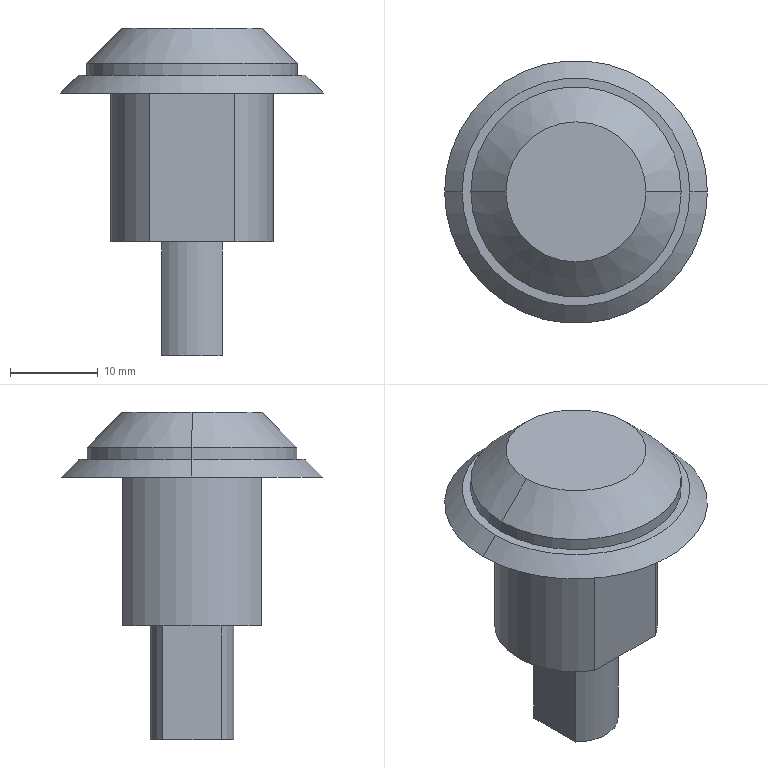Part | SolidWorks | features ICE 3, Chamfer 2, Extrusion 1 | 1 solid | 20 faces | box 30 x 30 x 37.4 mm | volume 8223 mm3 | plane 9 | cylinder 7 | cone 4 | commonest cylinder face diameters 18.6 x3 9.6 x2 24 x2
STEP:
#1=CARTESIAN_POINT('',(13.,0.,0.));
#2=VERTEX_POINT('',#1);
#3=CARTESIAN_POINT('',(-13.,0.,0.));
#4=VERTEX_POINT('',#3);
#5=CARTESIAN_POINT('',(0.,0.,0.));
#6=DIRECTION('',(0.,0.,1.));
#7=DIRECTION('',(-1.,0.,0.));
#8=AXIS2_PLACEMENT_3D('',#5,#6,#7);
#9=CIRCLE('',#8,13.);
#10=EDGE_CURVE('',#2,#4,#9,.T.);
#11=ORIENTED_EDGE('',*,*,#10,.F.);
#12=CARTESIAN_POINT('',(15.,0.,-2.));
#13=VERTEX_POINT('',#12);
#14=CARTESIAN_POINT('',(15.,0.,-2.));
#15=DIRECTION('',(0.7071,0.,-0.7071));
#16=VECTOR('',#15,1000.);
#17=LINE('',#14,#16);
#18=EDGE_CURVE('',#2,#13,#17,.T.);
#19=ORIENTED_EDGE('',*,*,#18,.T.);
#20=CARTESIAN_POINT('',(-15.,0.,-2.));
#21=VERTEX_POINT('',#20);
#22=CARTESIAN_POINT('',(0.,0.,-2.));
#23=DIRECTION('',(0.,0.,-1.));
#24=DIRECTION('',(-1.,0.,0.));
#25=AXIS2_PLACEMENT_3D('',#22,#23,#24);
#26=CIRCLE('',#25,15.);
#27=EDGE_CURVE('',#21,#13,#26,.T.);
#28=ORIENTED_EDGE('',*,*,#27,.F.);
#29=CARTESIAN_POINT('',(-15.,0.,-2.));
#30=DIRECTION('',(-0.7071,0.,-0.7071));
#31=VECTOR('',#30,1000.);
#32=LINE('',#29,#31);
#33=EDGE_CURVE('',#4,#21,#32,.T.);
#34=ORIENTED_EDGE('',*,*,#33,.F.);
#35=EDGE_LOOP('',(#11,#19,#28,#34));
#36=FACE_OUTER_BOUND('',#35,.T.);
#37=CARTESIAN_POINT('',(0.,0.,-2.));
#38=DIRECTION('',(0.,0.,-1.));
#39=DIRECTION('',(-1.,0.,0.));
#40=AXIS2_PLACEMENT_3D('',#37,#38,#39);
#41=CONICAL_SURFACE('',#40,15.,0.7854);
#42=ADVANCED_FACE('',(#36),#41,.T.);
#43=CARTESIAN_POINT('',(-12.,0.,1.4));
#44=VERTEX_POINT('',#43);
#45=CARTESIAN_POINT('',(12.,0.,1.4));
#46=VERTEX_POINT('',#45);
#47=CARTESIAN_POINT('',(0.,0.,1.4));
#48=DIRECTION('',(0.,0.,-1.));
#49=DIRECTION('',(1.,0.,0.));
#50=AXIS2_PLACEMENT_3D('',#47,#48,#49);
#51=CIRCLE('',#50,12.);
#52=EDGE_CURVE('',#44,#46,#51,.T.);
#53=ORIENTED_EDGE('',*,*,#52,.T.);
#54=CARTESIAN_POINT('',(12.,0.,0.));
#55=VERTEX_POINT('',#54);
#56=CARTESIAN_POINT('',(12.,0.,5.4));
#57=DIRECTION('',(0.,0.,-1.));
#58=VECTOR('',#57,1000.);
#59=LINE('',#56,#58);
#60=EDGE_CURVE('',#46,#55,#59,.T.);
#61=ORIENTED_EDGE('',*,*,#60,.T.);
#62=CARTESIAN_POINT('',(-12.,0.,0.));
#63=VERTEX_POINT('',#62);
#64=CARTESIAN_POINT('',(0.,0.,0.));
#65=DIRECTION('',(0.,0.,-1.));
#66=DIRECTION('',(-1.,0.,0.));
#67=AXIS2_PLACEMENT_3D('',#64,#65,#66);
#68=CIRCLE('',#67,12.);
#69=EDGE_CURVE('',#63,#55,#68,.T.);
#70=ORIENTED_EDGE('',*,*,#69,.F.);
#71=CARTESIAN_POINT('',(-12.,0.,5.4));
#72=DIRECTION('',(0.,0.,-1.));
#73=VECTOR('',#72,1000.);
#74=LINE('',#71,#73);
#75=EDGE_CURVE('',#44,#63,#74,.T.);
#76=ORIENTED_EDGE('',*,*,#75,.F.);
#77=EDGE_LOOP('',(#53,#61,#70,#76));
#78=FACE_OUTER_BOUND('',#77,.T.);
#79=CARTESIAN_POINT('',(0.,0.,5.4));
#80=DIRECTION('',(0.,0.,-1.));
#81=DIRECTION('',(-1.,0.,0.));
#82=AXIS2_PLACEMENT_3D('',#79,#80,#81);
#83=CYLINDRICAL_SURFACE('',#82,12.);
#84=ADVANCED_FACE('',(#78),#83,.T.);
#85=CARTESIAN_POINT('',(8.,0.,5.4));
#86=VERTEX_POINT('',#85);
#87=CARTESIAN_POINT('',(-8.,0.,5.4));
#88=VERTEX_POINT('',#87);
#89=CARTESIAN_POINT('',(0.,0.,5.4));
#90=DIRECTION('',(0.,0.,1.));
#91=DIRECTION('',(1.,0.,0.));
#92=AXIS2_PLACEMENT_3D('',#89,#90,#91);
#93=CIRCLE('',#92,8.);
#94=EDGE_CURVE('',#86,#88,#93,.T.);
#95=ORIENTED_EDGE('',*,*,#94,.F.);
#96=CARTESIAN_POINT('',(8.,0.,5.4));
#97=DIRECTION('',(0.7071,0.,-0.7071));
#98=VECTOR('',#97,1000.);
#99=LINE('',#96,#98);
#100=EDGE_CURVE('',#86,#46,#99,.T.);
#101=ORIENTED_EDGE('',*,*,#100,.T.);
#102=ORIENTED_EDGE('',*,*,#52,.F.);
#103=CARTESIAN_POINT('',(-8.,0.,5.4));
#104=DIRECTION('',(-0.7071,0.,-0.7071));
#105=VECTOR('',#104,1000.);
#106=LINE('',#103,#105);
#107=EDGE_CURVE('',#88,#44,#106,.T.);
#108=ORIENTED_EDGE('',*,*,#107,.F.);
#109=EDGE_LOOP('',(#95,#101,#102,#108));
#110=FACE_OUTER_BOUND('',#109,.T.);
#111=CARTESIAN_POINT('',(0.,0.,5.4));
#112=DIRECTION('',(0.,0.,-1.));
#113=DIRECTION('',(-1.,0.,0.));
#114=AXIS2_PLACEMENT_3D('',#111,#112,#113);
#115=CONICAL_SURFACE('',#114,8.,0.7854);
#116=ADVANCED_FACE('',(#110),#115,.T.);
#117=CARTESIAN_POINT('',(9.3,0.,-19.));
#118=VERTEX_POINT('',#117);
#119=CARTESIAN_POINT('',(4.907,-7.9,-19.));
#120=VERTEX_POINT('',#119);
#121=CARTESIAN_POINT('',(0.,0.,-19.));
#122=DIRECTION('',(0.,0.,-1.));
#123=DIRECTION('',(-1.,0.,0.));
#124=AXIS2_PLACEMENT_3D('',#121,#122,#123);
#125=CIRCLE('',#124,9.3);
#126=EDGE_CURVE('',#118,#120,#125,.T.);
#127=ORIENTED_EDGE('',*,*,#126,.F.);
#128=CARTESIAN_POINT('',(9.3,0.,-2.));
#129=VERTEX_POINT('',#128);
#130=CARTESIAN_POINT('',(9.3,0.,-19.));
#131=DIRECTION('',(0.,0.,1.));
#132=VECTOR('',#131,1000.);
#133=LINE('',#130,#132);
#134=EDGE_CURVE('',#118,#129,#133,.T.);
#135=ORIENTED_EDGE('',*,*,#134,.T.);
#136=CARTESIAN_POINT('',(4.907,-7.9,-2.));
#137=VERTEX_POINT('',#136);
#138=CARTESIAN_POINT('',(0.,0.,-2.));
#139=DIRECTION('',(0.,0.,-1.));
#140=DIRECTION('',(-1.,0.,0.));
#141=AXIS2_PLACEMENT_3D('',#138,#139,#140);
#142=CIRCLE('',#141,9.3);
#143=EDGE_CURVE('',#129,#137,#142,.T.);
#144=ORIENTED_EDGE('',*,*,#143,.T.);
#145=CARTESIAN_POINT('',(4.907,-7.9,-19.));
#146=DIRECTION('',(0.,0.,1.));
#147=VECTOR('',#146,1000.);
#148=LINE('',#145,#147);
#149=EDGE_CURVE('',#120,#137,#148,.T.);
#150=ORIENTED_EDGE('',*,*,#149,.F.);
#151=EDGE_LOOP('',(#127,#135,#144,#150));
#152=FACE_OUTER_BOUND('',#151,.T.);
#153=CARTESIAN_POINT('',(0.,0.,-19.));
#154=DIRECTION('',(0.,0.,1.));
#155=DIRECTION('',(1.,0.,0.));
#156=AXIS2_PLACEMENT_3D('',#153,#154,#155);
#157=CYLINDRICAL_SURFACE('',#156,9.3);
#158=ADVANCED_FACE('',(#152),#157,.T.);
#159=CARTESIAN_POINT('',(-4.907,-7.9,-19.));
#160=VERTEX_POINT('',#159);
#161=CARTESIAN_POINT('',(-4.907,7.9,-19.));
#162=VERTEX_POINT('',#161);
#163=CARTESIAN_POINT('',(0.,0.,-19.));
#164=DIRECTION('',(0.,0.,-1.));
#165=DIRECTION('',(-1.,0.,0.));
#166=AXIS2_PLACEMENT_3D('',#163,#164,#165);
#167=CIRCLE('',#166,9.3);
#168=EDGE_CURVE('',#160,#162,#167,.T.);
#169=ORIENTED_EDGE('',*,*,#168,.T.);
#170=CARTESIAN_POINT('',(4.907,7.9,-19.));
#171=VERTEX_POINT('',#170);
#172=CARTESIAN_POINT('',(4.907,7.9,-19.));
#173=DIRECTION('',(1.,0.,0.));
#174=VECTOR('',#173,1000.);
#175=LINE('',#172,#174);
#176=EDGE_CURVE('',#162,#171,#175,.T.);
#177=ORIENTED_EDGE('',*,*,#176,.T.);
#178=CARTESIAN_POINT('',(0.,0.,-19.));
#179=DIRECTION('',(0.,0.,-1.));
#180=DIRECTION('',(-1.,0.,0.));
#181=AXIS2_PLACEMENT_3D('',#178,#179,#180);
#182=CIRCLE('',#181,9.3);
#183=EDGE_CURVE('',#171,#118,#182,.T.);
#184=ORIENTED_EDGE('',*,*,#183,.T.);
#185=ORIENTED_EDGE('',*,*,#126,.T.);
#186=CARTESIAN_POINT('',(4.907,-7.9,-19.));
#187=DIRECTION('',(-1.,0.,0.));
#188=VECTOR('',#187,1000.);
#189=LINE('',#186,#188);
#190=EDGE_CURVE('',#120,#160,#189,.T.);
#191=ORIENTED_EDGE('',*,*,#190,.T.);
#192=EDGE_LOOP('',(#169,#177,#184,#185,#191));
#193=FACE_OUTER_BOUND('',#192,.T.);
#194=CARTESIAN_POINT('',(-3.45,-3.337,-19.));
#195=VERTEX_POINT('',#194);
#196=CARTESIAN_POINT('',(-3.45,3.337,-19.));
#197=VERTEX_POINT('',#196);
#198=CARTESIAN_POINT('',(-3.45,-3.337,-19.));
#199=DIRECTION('',(0.,1.,0.));
#200=VECTOR('',#199,1000.);
#201=LINE('',#198,#200);
#202=EDGE_CURVE('',#195,#197,#201,.T.);
#203=ORIENTED_EDGE('',*,*,#202,.F.);
#204=CARTESIAN_POINT('',(3.45,-3.337,-19.));
#205=VERTEX_POINT('',#204);
#206=CARTESIAN_POINT('',(0.,0.,-19.));
#207=DIRECTION('',(0.,0.,-1.));
#208=DIRECTION('',(-1.,0.,0.));
#209=AXIS2_PLACEMENT_3D('',#206,#207,#208);
#210=CIRCLE('',#209,4.8);
#211=EDGE_CURVE('',#205,#195,#210,.T.);
#212=ORIENTED_EDGE('',*,*,#211,.F.);
#213=CARTESIAN_POINT('',(3.45,3.337,-19.));
#214=VERTEX_POINT('',#213);
#215=CARTESIAN_POINT('',(3.45,-3.337,-19.));
#216=DIRECTION('',(0.,-1.,0.));
#217=VECTOR('',#216,1000.);
#218=LINE('',#215,#217);
#219=EDGE_CURVE('',#214,#205,#218,.T.);
#220=ORIENTED_EDGE('',*,*,#219,.F.);
#221=CARTESIAN_POINT('',(0.,0.,-19.));
#222=DIRECTION('',(0.,0.,-1.));
#223=DIRECTION('',(-1.,0.,0.));
#224=AXIS2_PLACEMENT_3D('',#221,#222,#223);
#225=CIRCLE('',#224,4.8);
#226=EDGE_CURVE('',#197,#214,#225,.T.);
#227=ORIENTED_EDGE('',*,*,#226,.F.);
#228=EDGE_LOOP('',(#203,#212,#220,#227));
#229=FACE_BOUND('',#228,.T.);
#230=CARTESIAN_POINT('',(0.,0.,-19.));
#231=DIRECTION('',(0.,0.,-1.));
#232=DIRECTION('',(-1.,0.,0.));
#233=AXIS2_PLACEMENT_3D('',#230,#231,#232);
#234=PLANE('',#233);
#235=ADVANCED_FACE('',(#193,#229),#234,.T.);
#236=CARTESIAN_POINT('',(-4.907,-7.9,-2.));
#237=VERTEX_POINT('',#236);
#238=CARTESIAN_POINT('',(-4.907,-7.9,-19.));
#239=DIRECTION('',(0.,0.,1.));
#240=VECTOR('',#239,1000.);
#241=LINE('',#238,#240);
#242=EDGE_CURVE('',#160,#237,#241,.T.);
#243=ORIENTED_EDGE('',*,*,#242,.T.);
#244=CARTESIAN_POINT('',(-4.907,7.9,-2.));
#245=VERTEX_POINT('',#244);
#246=CARTESIAN_POINT('',(0.,0.,-2.));
#247=DIRECTION('',(0.,0.,-1.));
#248=DIRECTION('',(-1.,0.,0.));
#249=AXIS2_PLACEMENT_3D('',#246,#247,#248);
#250=CIRCLE('',#249,9.3);
#251=EDGE_CURVE('',#237,#245,#250,.T.);
#252=ORIENTED_EDGE('',*,*,#251,.T.);
#253=CARTESIAN_POINT('',(-4.907,7.9,-19.));
#254=DIRECTION('',(0.,0.,1.));
#255=VECTOR('',#254,1000.);
#256=LINE('',#253,#255);
#257=EDGE_CURVE('',#162,#245,#256,.T.);
#258=ORIENTED_EDGE('',*,*,#257,.F.);
#259=ORIENTED_EDGE('',*,*,#168,.F.);
#260=EDGE_LOOP('',(#243,#252,#258,#259));
#261=FACE_OUTER_BOUND('',#260,.T.);
#262=CARTESIAN_POINT('',(0.,0.,-19.));
#263=DIRECTION('',(0.,0.,1.));
#264=DIRECTION('',(1.,0.,0.));
#265=AXIS2_PLACEMENT_3D('',#262,#263,#264);
#266=CYLINDRICAL_SURFACE('',#265,9.3);
#267=ADVANCED_FACE('',(#261),#266,.T.);
#268=ORIENTED_EDGE('',*,*,#257,.T.);
#269=CARTESIAN_POINT('',(4.907,7.9,-2.));
#270=VERTEX_POINT('',#269);
#271=CARTESIAN_POINT('',(4.907,7.9,-2.));
#272=DIRECTION('',(1.,0.,0.));
#273=VECTOR('',#272,1000.);
#274=LINE('',#271,#273);
#275=EDGE_CURVE('',#245,#270,#274,.T.);
#276=ORIENTED_EDGE('',*,*,#275,.T.);
#277=CARTESIAN_POINT('',(4.907,7.9,-19.));
#278=DIRECTION('',(0.,0.,1.));
#279=VECTOR('',#278,1000.);
#280=LINE('',#277,#279);
#281=EDGE_CURVE('',#171,#270,#280,.T.);
#282=ORIENTED_EDGE('',*,*,#281,.F.);
#283=ORIENTED_EDGE('',*,*,#176,.F.);
#284=EDGE_LOOP('',(#268,#276,#282,#283));
#285=FACE_OUTER_BOUND('',#284,.T.);
#286=CARTESIAN_POINT('',(4.907,7.9,-19.));
#287=DIRECTION('',(0.,-1.,0.));
#288=DIRECTION('',(0.,0.,-1.));
#289=AXIS2_PLACEMENT_3D('',#286,#287,#288);
#290=PLANE('',#289);
#291=ADVANCED_FACE('',(#285),#290,.F.);
#292=ORIENTED_EDGE('',*,*,#134,.F.);
#293=ORIENTED_EDGE('',*,*,#183,.F.);
#294=ORIENTED_EDGE('',*,*,#281,.T.);
#295=CARTESIAN_POINT('',(0.,0.,-2.));
#296=DIRECTION('',(0.,0.,-1.));
#297=DIRECTION('',(-1.,0.,0.));
#298=AXIS2_PLACEMENT_3D('',#295,#296,#297);
#299=CIRCLE('',#298,9.3);
#300=EDGE_CURVE('',#270,#129,#299,.T.);
#301=ORIENTED_EDGE('',*,*,#300,.T.);
#302=EDGE_LOOP('',(#292,#293,#294,#301));
#303=FACE_OUTER_BOUND('',#302,.T.);
#304=CARTESIAN_POINT('',(0.,0.,-19.));
#305=DIRECTION('',(0.,0.,1.));
#306=DIRECTION('',(1.,0.,0.));
#307=AXIS2_PLACEMENT_3D('',#304,#305,#306);
#308=CYLINDRICAL_SURFACE('',#307,9.3);
#309=ADVANCED_FACE('',(#303),#308,.T.);
#310=ORIENTED_EDGE('',*,*,#149,.T.);
#311=CARTESIAN_POINT('',(4.907,-7.9,-2.));
#312=DIRECTION('',(-1.,0.,0.));
#313=VECTOR('',#312,1000.);
#314=LINE('',#311,#313);
#315=EDGE_CURVE('',#137,#237,#314,.T.);
#316=ORIENTED_EDGE('',*,*,#315,.T.);
#317=ORIENTED_EDGE('',*,*,#242,.F.);
#318=ORIENTED_EDGE('',*,*,#190,.F.);
#319=EDGE_LOOP('',(#310,#316,#317,#318));
#320=FACE_OUTER_BOUND('',#319,.T.);
#321=CARTESIAN_POINT('',(4.907,-7.9,-19.));
#322=DIRECTION('',(0.,1.,0.));
#323=DIRECTION('',(0.,0.,1.));
#324=AXIS2_PLACEMENT_3D('',#321,#322,#323);
#325=PLANE('',#324);
#326=ADVANCED_FACE('',(#320),#325,.F.);
#327=ORIENTED_EDGE('',*,*,#211,.T.);
#328=CARTESIAN_POINT('',(-3.45,-3.337,-32.));
#329=VERTEX_POINT('',#328);
#330=CARTESIAN_POINT('',(-3.45,-3.337,-32.));
#331=DIRECTION('',(0.,0.,1.));
#332=VECTOR('',#331,1000.);
#333=LINE('',#330,#332);
#334=EDGE_CURVE('',#329,#195,#333,.T.);
#335=ORIENTED_EDGE('',*,*,#334,.F.);
#336=CARTESIAN_POINT('',(3.45,-3.337,-32.));
#337=VERTEX_POINT('',#336);
#338=CARTESIAN_POINT('',(0.,0.,-32.));
#339=DIRECTION('',(0.,0.,-1.));
#340=DIRECTION('',(-1.,0.,0.));
#341=AXIS2_PLACEMENT_3D('',#338,#339,#340);
#342=CIRCLE('',#341,4.8);
#343=EDGE_CURVE('',#337,#329,#342,.T.);
#344=ORIENTED_EDGE('',*,*,#343,.F.);
#345=CARTESIAN_POINT('',(3.45,-3.337,-32.));
#346=DIRECTION('',(0.,0.,1.));
#347=VECTOR('',#346,1000.);
#348=LINE('',#345,#347);
#349=EDGE_CURVE('',#337,#205,#348,.T.);
#350=ORIENTED_EDGE('',*,*,#349,.T.);
#351=EDGE_LOOP('',(#327,#335,#344,#350));
#352=FACE_OUTER_BOUND('',#351,.T.);
#353=CARTESIAN_POINT('',(0.,0.,-32.));
#354=DIRECTION('',(0.,0.,1.));
#355=DIRECTION('',(1.,0.,0.));
#356=AXIS2_PLACEMENT_3D('',#353,#354,#355);
#357=CYLINDRICAL_SURFACE('',#356,4.8);
#358=ADVANCED_FACE('',(#352),#357,.T.);
#359=ORIENTED_EDGE('',*,*,#202,.T.);
#360=CARTESIAN_POINT('',(-3.45,3.337,-32.));
#361=VERTEX_POINT('',#360);
#362=CARTESIAN_POINT('',(-3.45,3.337,-32.));
#363=DIRECTION('',(0.,0.,1.));
#364=VECTOR('',#363,1000.);
#365=LINE('',#362,#364);
#366=EDGE_CURVE('',#361,#197,#365,.T.);
#367=ORIENTED_EDGE('',*,*,#366,.F.);
#368=CARTESIAN_POINT('',(-3.45,-3.337,-32.));
#369=DIRECTION('',(0.,1.,0.));
#370=VECTOR('',#369,1000.);
#371=LINE('',#368,#370);
#372=EDGE_CURVE('',#329,#361,#371,.T.);
#373=ORIENTED_EDGE('',*,*,#372,.F.);
#374=ORIENTED_EDGE('',*,*,#334,.T.);
#375=EDGE_LOOP('',(#359,#367,#373,#374));
#376=FACE_OUTER_BOUND('',#375,.T.);
#377=CARTESIAN_POINT('',(-3.45,-3.337,-32.));
#378=DIRECTION('',(1.,0.,0.));
#379=DIRECTION('',(0.,1.,0.));
#380=AXIS2_PLACEMENT_3D('',#377,#378,#379);
#381=PLANE('',#380);
#382=ADVANCED_FACE('',(#376),#381,.F.);
#383=ORIENTED_EDGE('',*,*,#226,.T.);
#384=CARTESIAN_POINT('',(3.45,3.337,-32.));
#385=VERTEX_POINT('',#384);
#386=CARTESIAN_POINT('',(3.45,3.337,-32.));
#387=DIRECTION('',(0.,0.,1.));
#388=VECTOR('',#387,1000.);
#389=LINE('',#386,#388);
#390=EDGE_CURVE('',#385,#214,#389,.T.);
#391=ORIENTED_EDGE('',*,*,#390,.F.);
#392=CARTESIAN_POINT('',(0.,0.,-32.));
#393=DIRECTION('',(0.,0.,-1.));
#394=DIRECTION('',(-1.,0.,0.));
#395=AXIS2_PLACEMENT_3D('',#392,#393,#394);
#396=CIRCLE('',#395,4.8);
#397=EDGE_CURVE('',#361,#385,#396,.T.);
#398=ORIENTED_EDGE('',*,*,#397,.F.);
#399=ORIENTED_EDGE('',*,*,#366,.T.);
#400=EDGE_LOOP('',(#383,#391,#398,#399));
#401=FACE_OUTER_BOUND('',#400,.T.);
#402=CARTESIAN_POINT('',(0.,0.,-32.));
#403=DIRECTION('',(0.,0.,1.));
#404=DIRECTION('',(1.,0.,0.));
#405=AXIS2_PLACEMENT_3D('',#402,#403,#404);
#406=CYLINDRICAL_SURFACE('',#405,4.8);
#407=ADVANCED_FACE('',(#401),#406,.T.);
#408=ORIENTED_EDGE('',*,*,#219,.T.);
#409=ORIENTED_EDGE('',*,*,#349,.F.);
#410=CARTESIAN_POINT('',(3.45,-3.337,-32.));
#411=DIRECTION('',(0.,-1.,0.));
#412=VECTOR('',#411,1000.);
#413=LINE('',#410,#412);
#414=EDGE_CURVE('',#385,#337,#413,.T.);
#415=ORIENTED_EDGE('',*,*,#414,.F.);
#416=ORIENTED_EDGE('',*,*,#390,.T.);
#417=EDGE_LOOP('',(#408,#409,#415,#416));
#418=FACE_OUTER_BOUND('',#417,.T.);
#419=CARTESIAN_POINT('',(3.45,-3.337,-32.));
#420=DIRECTION('',(-1.,0.,0.));
#421=DIRECTION('',(0.,-1.,0.));
#422=AXIS2_PLACEMENT_3D('',#419,#420,#421);
#423=PLANE('',#422);
#424=ADVANCED_FACE('',(#418),#423,.F.);
#425=ORIENTED_EDGE('',*,*,#343,.T.);
#426=ORIENTED_EDGE('',*,*,#372,.T.);
#427=ORIENTED_EDGE('',*,*,#397,.T.);
#428=ORIENTED_EDGE('',*,*,#414,.T.);
#429=EDGE_LOOP('',(#425,#426,#427,#428));
#430=FACE_OUTER_BOUND('',#429,.T.);
#431=CARTESIAN_POINT('',(0.,0.,-32.));
#432=DIRECTION('',(0.,0.,-1.));
#433=DIRECTION('',(-1.,0.,0.));
#434=AXIS2_PLACEMENT_3D('',#431,#432,#433);
#435=PLANE('',#434);
#436=ADVANCED_FACE('',(#430),#435,.T.);
#437=ORIENTED_EDGE('',*,*,#27,.T.);
#438=CARTESIAN_POINT('',(0.,0.,-2.));
#439=DIRECTION('',(0.,0.,-1.));
#440=DIRECTION('',(-1.,0.,0.));
#441=AXIS2_PLACEMENT_3D('',#438,#439,#440);
#442=CIRCLE('',#441,15.);
#443=EDGE_CURVE('',#13,#21,#442,.T.);
#444=ORIENTED_EDGE('',*,*,#443,.T.);
#445=EDGE_LOOP('',(#437,#444));
#446=FACE_OUTER_BOUND('',#445,.T.);
#447=ORIENTED_EDGE('',*,*,#251,.F.);
#448=ORIENTED_EDGE('',*,*,#315,.F.);
#449=ORIENTED_EDGE('',*,*,#143,.F.);
#450=ORIENTED_EDGE('',*,*,#300,.F.);
#451=ORIENTED_EDGE('',*,*,#275,.F.);
#452=EDGE_LOOP('',(#447,#448,#449,#450,#451));
#453=FACE_BOUND('',#452,.T.);
#454=CARTESIAN_POINT('',(0.,0.,-2.));
#455=DIRECTION('',(0.,0.,-1.));
#456=DIRECTION('',(-1.,0.,0.));
#457=AXIS2_PLACEMENT_3D('',#454,#455,#456);
#458=PLANE('',#457);
#459=ADVANCED_FACE('',(#446,#453),#458,.T.);
#460=CARTESIAN_POINT('',(0.,0.,0.));
#461=DIRECTION('',(0.,0.,1.));
#462=DIRECTION('',(-1.,0.,0.));
#463=AXIS2_PLACEMENT_3D('',#460,#461,#462);
#464=CIRCLE('',#463,13.);
#465=EDGE_CURVE('',#4,#2,#464,.T.);
#466=ORIENTED_EDGE('',*,*,#465,.T.);
#467=ORIENTED_EDGE('',*,*,#10,.T.);
#468=EDGE_LOOP('',(#466,#467));
#469=FACE_OUTER_BOUND('',#468,.T.);
#470=ORIENTED_EDGE('',*,*,#69,.T.);
#471=CARTESIAN_POINT('',(0.,0.,0.));
#472=DIRECTION('',(0.,0.,-1.));
#473=DIRECTION('',(-1.,0.,0.));
#474=AXIS2_PLACEMENT_3D('',#471,#472,#473);
#475=CIRCLE('',#474,12.);
#476=EDGE_CURVE('',#55,#63,#475,.T.);
#477=ORIENTED_EDGE('',*,*,#476,.T.);
#478=EDGE_LOOP('',(#470,#477));
#479=FACE_BOUND('',#478,.T.);
#480=CARTESIAN_POINT('',(0.,0.,0.));
#481=DIRECTION('',(0.,0.,-1.));
#482=DIRECTION('',(-1.,0.,0.));
#483=AXIS2_PLACEMENT_3D('',#480,#481,#482);
#484=PLANE('',#483);
#485=ADVANCED_FACE('',(#469,#479),#484,.F.);
#486=CARTESIAN_POINT('',(0.,0.,5.4));
#487=DIRECTION('',(0.,0.,1.));
#488=DIRECTION('',(1.,0.,0.));
#489=AXIS2_PLACEMENT_3D('',#486,#487,#488);
#490=CIRCLE('',#489,8.);
#491=EDGE_CURVE('',#88,#86,#490,.T.);
#492=ORIENTED_EDGE('',*,*,#491,.T.);
#493=ORIENTED_EDGE('',*,*,#94,.T.);
#494=EDGE_LOOP('',(#492,#493));
#495=FACE_OUTER_BOUND('',#494,.T.);
#496=CARTESIAN_POINT('',(0.,0.,5.4));
#497=DIRECTION('',(0.,0.,1.));
#498=DIRECTION('',(1.,0.,0.));
#499=AXIS2_PLACEMENT_3D('',#496,#497,#498);
#500=PLANE('',#499);
#501=ADVANCED_FACE('',(#495),#500,.T.);
#502=ORIENTED_EDGE('',*,*,#100,.F.);
#503=ORIENTED_EDGE('',*,*,#491,.F.);
#504=ORIENTED_EDGE('',*,*,#107,.T.);
#505=CARTESIAN_POINT('',(0.,0.,1.4));
#506=DIRECTION('',(0.,0.,-1.));
#507=DIRECTION('',(1.,0.,0.));
#508=AXIS2_PLACEMENT_3D('',#505,#506,#507);
#509=CIRCLE('',#508,12.);
#510=EDGE_CURVE('',#46,#44,#509,.T.);
#511=ORIENTED_EDGE('',*,*,#510,.F.);
#512=EDGE_LOOP('',(#502,#503,#504,#511));
#513=FACE_OUTER_BOUND('',#512,.T.);
#514=CARTESIAN_POINT('',(0.,0.,5.4));
#515=DIRECTION('',(0.,0.,-1.));
#516=DIRECTION('',(-1.,0.,0.));
#517=AXIS2_PLACEMENT_3D('',#514,#515,#516);
#518=CONICAL_SURFACE('',#517,8.,0.7854);
#519=ADVANCED_FACE('',(#513),#518,.T.);
#520=ORIENTED_EDGE('',*,*,#60,.F.);
#521=ORIENTED_EDGE('',*,*,#510,.T.);
#522=ORIENTED_EDGE('',*,*,#75,.T.);
#523=ORIENTED_EDGE('',*,*,#476,.F.);
#524=EDGE_LOOP('',(#520,#521,#522,#523));
#525=FACE_OUTER_BOUND('',#524,.T.);
#526=CARTESIAN_POINT('',(0.,0.,5.4));
#527=DIRECTION('',(0.,0.,-1.));
#528=DIRECTION('',(-1.,0.,0.));
#529=AXIS2_PLACEMENT_3D('',#526,#527,#528);
#530=CYLINDRICAL_SURFACE('',#529,12.);
#531=ADVANCED_FACE('',(#525),#530,.T.);
#532=ORIENTED_EDGE('',*,*,#18,.F.);
#533=ORIENTED_EDGE('',*,*,#465,.F.);
#534=ORIENTED_EDGE('',*,*,#33,.T.);
#535=ORIENTED_EDGE('',*,*,#443,.F.);
#536=EDGE_LOOP('',(#532,#533,#534,#535));
#537=FACE_OUTER_BOUND('',#536,.T.);
#538=CARTESIAN_POINT('',(0.,0.,-2.));
#539=DIRECTION('',(0.,0.,-1.));
#540=DIRECTION('',(-1.,0.,0.));
#541=AXIS2_PLACEMENT_3D('',#538,#539,#540);
#542=CONICAL_SURFACE('',#541,15.,0.7854);
#543=ADVANCED_FACE('',(#537),#542,.T.);
#544=CLOSED_SHELL('',(#42,#84,#116,#158,#235,#267,#291,#309,#326,#358,#382,#407,#424,#436,#459,#485,#501,#519,#531,#543));
#545=MANIFOLD_SOLID_BREP('',#544);
#546=CARTESIAN_POINT('',(0.,0.,0.));
#547=DIRECTION('',(0.,0.,1.));
#548=DIRECTION('',(1.,0.,0.));
#549=AXIS2_PLACEMENT_3D('',#546,#547,#548);
#550=(LENGTH_UNIT()NAMED_UNIT(*)SI_UNIT(.MILLI.,.METRE.));
#551=UNCERTAINTY_MEASURE_WITH_UNIT(LENGTH_MEASURE(0.00001),#550,'','');
#552=(NAMED_UNIT(*)PLANE_ANGLE_UNIT()SI_UNIT($,.RADIAN.));
#553=(NAMED_UNIT(*)SI_UNIT($,.STERADIAN.)SOLID_ANGLE_UNIT());
#554=(GEOMETRIC_REPRESENTATION_CONTEXT(3)GLOBAL_UNCERTAINTY_ASSIGNED_CONTEXT((#551))GLOBAL_UNIT_ASSIGNED_CONTEXT((#550,#552,#553))REPRESENTATION_CONTEXT('',''));
#555=ADVANCED_BREP_SHAPE_REPRESENTATION('',(#545,#549),#554);